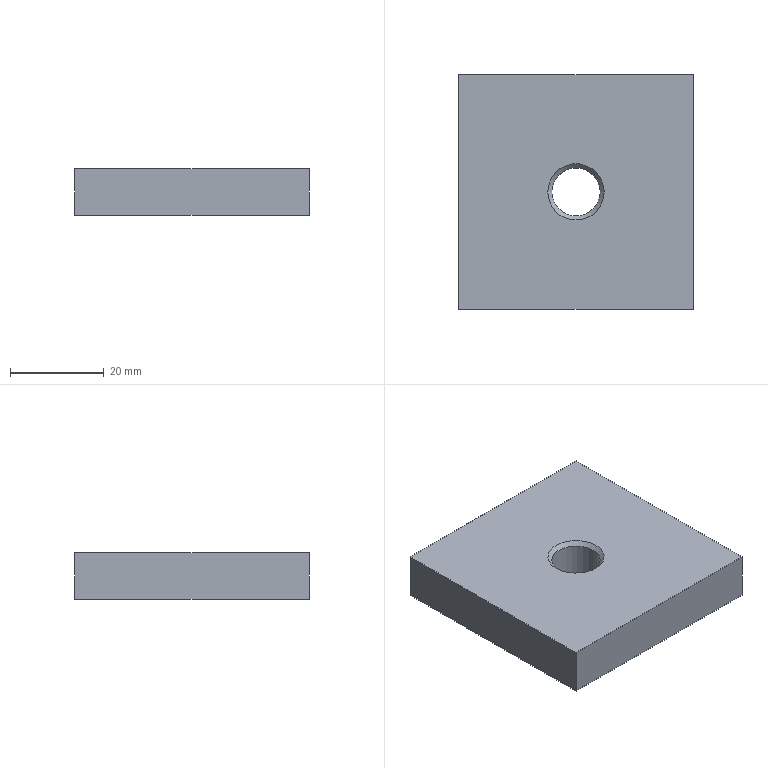Part | STEP file | 冲床-300配套压波_id898_x_t | 1 solid | 9 faces | box 50 x 50 x 10 mm | volume 24142 mm3 | plane 6 | cone 2 | cylinder 1 | commonest cylinder face diameters 10.3 x1
STEP:
#1=CARTESIAN_POINT('',(1160.,230.,-780.));
#2=VERTEX_POINT('',#1);
#3=CARTESIAN_POINT('',(1160.,280.,-780.));
#4=VERTEX_POINT('',#3);
#5=CARTESIAN_POINT('',(1160.,230.,-780.));
#6=DIRECTION('',(0.,1.,0.));
#7=VECTOR('',#6,1.);
#8=LINE('',#5,#7);
#9=EDGE_CURVE('',#2,#4,#8,.T.);
#10=ORIENTED_EDGE('',*,*,#9,.T.);
#11=CARTESIAN_POINT('',(1160.,280.,-790.));
#12=VERTEX_POINT('',#11);
#13=CARTESIAN_POINT('',(1160.,280.,-790.));
#14=DIRECTION('',(0.,0.,1.));
#15=VECTOR('',#14,1.);
#16=LINE('',#13,#15);
#17=EDGE_CURVE('',#12,#4,#16,.T.);
#18=ORIENTED_EDGE('',*,*,#17,.F.);
#19=CARTESIAN_POINT('',(1160.,230.,-790.));
#20=VERTEX_POINT('',#19);
#21=CARTESIAN_POINT('',(1160.,230.,-790.));
#22=DIRECTION('',(0.,1.,0.));
#23=VECTOR('',#22,1.);
#24=LINE('',#21,#23);
#25=EDGE_CURVE('',#20,#12,#24,.T.);
#26=ORIENTED_EDGE('',*,*,#25,.F.);
#27=CARTESIAN_POINT('',(1160.,230.,-790.));
#28=DIRECTION('',(0.,0.,1.));
#29=VECTOR('',#28,1.);
#30=LINE('',#27,#29);
#31=EDGE_CURVE('',#20,#2,#30,.T.);
#32=ORIENTED_EDGE('',*,*,#31,.T.);
#33=EDGE_LOOP('',(#10,#18,#26,#32));
#34=FACE_OUTER_BOUND('',#33,.T.);
#35=CARTESIAN_POINT('',(1160.,230.,-790.));
#36=DIRECTION('',(1.,0.,0.));
#37=DIRECTION('',(0.,0.,1.));
#38=AXIS2_PLACEMENT_3D('',#35,#36,#37);
#39=PLANE('',#38);
#40=ADVANCED_FACE('',(#34),#39,.F.);
#41=CARTESIAN_POINT('',(1210.,280.,-780.));
#42=VERTEX_POINT('',#41);
#43=CARTESIAN_POINT('',(1160.,280.,-780.));
#44=DIRECTION('',(1.,0.,0.));
#45=VECTOR('',#44,1.);
#46=LINE('',#43,#45);
#47=EDGE_CURVE('',#4,#42,#46,.T.);
#48=ORIENTED_EDGE('',*,*,#47,.T.);
#49=CARTESIAN_POINT('',(1210.,280.,-790.));
#50=VERTEX_POINT('',#49);
#51=CARTESIAN_POINT('',(1210.,280.,-790.));
#52=DIRECTION('',(0.,0.,1.));
#53=VECTOR('',#52,1.);
#54=LINE('',#51,#53);
#55=EDGE_CURVE('',#50,#42,#54,.T.);
#56=ORIENTED_EDGE('',*,*,#55,.F.);
#57=CARTESIAN_POINT('',(1160.,280.,-790.));
#58=DIRECTION('',(1.,0.,0.));
#59=VECTOR('',#58,1.);
#60=LINE('',#57,#59);
#61=EDGE_CURVE('',#12,#50,#60,.T.);
#62=ORIENTED_EDGE('',*,*,#61,.F.);
#63=ORIENTED_EDGE('',*,*,#17,.T.);
#64=EDGE_LOOP('',(#48,#56,#62,#63));
#65=FACE_OUTER_BOUND('',#64,.T.);
#66=CARTESIAN_POINT('',(1160.,280.,-790.));
#67=DIRECTION('',(0.,-1.,0.));
#68=DIRECTION('',(0.,0.,-1.));
#69=AXIS2_PLACEMENT_3D('',#66,#67,#68);
#70=PLANE('',#69);
#71=ADVANCED_FACE('',(#65),#70,.F.);
#72=CARTESIAN_POINT('',(1210.,230.,-780.));
#73=VERTEX_POINT('',#72);
#74=CARTESIAN_POINT('',(1210.,280.,-780.));
#75=DIRECTION('',(0.,-1.,0.));
#76=VECTOR('',#75,1.);
#77=LINE('',#74,#76);
#78=EDGE_CURVE('',#42,#73,#77,.T.);
#79=ORIENTED_EDGE('',*,*,#78,.T.);
#80=CARTESIAN_POINT('',(1210.,230.,-790.));
#81=VERTEX_POINT('',#80);
#82=CARTESIAN_POINT('',(1210.,230.,-790.));
#83=DIRECTION('',(0.,0.,1.));
#84=VECTOR('',#83,1.);
#85=LINE('',#82,#84);
#86=EDGE_CURVE('',#81,#73,#85,.T.);
#87=ORIENTED_EDGE('',*,*,#86,.F.);
#88=CARTESIAN_POINT('',(1210.,280.,-790.));
#89=DIRECTION('',(0.,-1.,0.));
#90=VECTOR('',#89,1.);
#91=LINE('',#88,#90);
#92=EDGE_CURVE('',#50,#81,#91,.T.);
#93=ORIENTED_EDGE('',*,*,#92,.F.);
#94=ORIENTED_EDGE('',*,*,#55,.T.);
#95=EDGE_LOOP('',(#79,#87,#93,#94));
#96=FACE_OUTER_BOUND('',#95,.T.);
#97=CARTESIAN_POINT('',(1210.,280.,-790.));
#98=DIRECTION('',(-1.,0.,0.));
#99=DIRECTION('',(0.,0.,-1.));
#100=AXIS2_PLACEMENT_3D('',#97,#98,#99);
#101=PLANE('',#100);
#102=ADVANCED_FACE('',(#96),#101,.F.);
#103=CARTESIAN_POINT('',(1210.,230.,-780.));
#104=DIRECTION('',(-1.,0.,0.));
#105=VECTOR('',#104,1.);
#106=LINE('',#103,#105);
#107=EDGE_CURVE('',#73,#2,#106,.T.);
#108=ORIENTED_EDGE('',*,*,#107,.T.);
#109=ORIENTED_EDGE('',*,*,#31,.F.);
#110=CARTESIAN_POINT('',(1210.,230.,-790.));
#111=DIRECTION('',(-1.,0.,0.));
#112=VECTOR('',#111,1.);
#113=LINE('',#110,#112);
#114=EDGE_CURVE('',#81,#20,#113,.T.);
#115=ORIENTED_EDGE('',*,*,#114,.F.);
#116=ORIENTED_EDGE('',*,*,#86,.T.);
#117=EDGE_LOOP('',(#108,#109,#115,#116));
#118=FACE_OUTER_BOUND('',#117,.T.);
#119=CARTESIAN_POINT('',(1210.,230.,-790.));
#120=DIRECTION('',(0.,1.,0.));
#121=DIRECTION('',(1.,0.,0.));
#122=AXIS2_PLACEMENT_3D('',#119,#120,#121);
#123=PLANE('',#122);
#124=ADVANCED_FACE('',(#118),#123,.F.);
#125=CARTESIAN_POINT('',(1179.,255.,-790.));
#126=VERTEX_POINT('',#125);
#127=CARTESIAN_POINT('',(1185.,255.,-790.));
#128=DIRECTION('',(0.,0.,1.));
#129=DIRECTION('',(-1.,0.,0.));
#130=AXIS2_PLACEMENT_3D('',#127,#128,#129);
#131=CIRCLE('',#130,6.);
#132=EDGE_CURVE('',#126,#126,#131,.T.);
#133=ORIENTED_EDGE('',*,*,#132,.T.);
#134=EDGE_LOOP('',(#133));
#135=FACE_BOUND('',#134,.T.);
#136=ORIENTED_EDGE('',*,*,#25,.T.);
#137=ORIENTED_EDGE('',*,*,#61,.T.);
#138=ORIENTED_EDGE('',*,*,#92,.T.);
#139=ORIENTED_EDGE('',*,*,#114,.T.);
#140=EDGE_LOOP('',(#136,#137,#138,#139));
#141=FACE_BOUND('',#140,.T.);
#142=CARTESIAN_POINT('',(10.,480.,-790.));
#143=DIRECTION('',(0.,0.,-1.));
#144=DIRECTION('',(1.,0.,0.));
#145=AXIS2_PLACEMENT_3D('',#142,#143,#144);
#146=PLANE('',#145);
#147=ADVANCED_FACE('',(#135,#141),#146,.T.);
#148=CARTESIAN_POINT('',(1179.,255.,-780.));
#149=VERTEX_POINT('',#148);
#150=CARTESIAN_POINT('',(1185.,255.,-780.));
#151=DIRECTION('',(0.,0.,-1.));
#152=DIRECTION('',(-1.,0.,0.));
#153=AXIS2_PLACEMENT_3D('',#150,#151,#152);
#154=CIRCLE('',#153,6.);
#155=EDGE_CURVE('',#149,#149,#154,.T.);
#156=ORIENTED_EDGE('',*,*,#155,.T.);
#157=EDGE_LOOP('',(#156));
#158=FACE_BOUND('',#157,.T.);
#159=ORIENTED_EDGE('',*,*,#9,.F.);
#160=ORIENTED_EDGE('',*,*,#107,.F.);
#161=ORIENTED_EDGE('',*,*,#78,.F.);
#162=ORIENTED_EDGE('',*,*,#47,.F.);
#163=EDGE_LOOP('',(#159,#160,#161,#162));
#164=FACE_BOUND('',#163,.T.);
#165=CARTESIAN_POINT('',(10.,480.,-780.));
#166=DIRECTION('',(0.,0.,-1.));
#167=DIRECTION('',(1.,0.,0.));
#168=AXIS2_PLACEMENT_3D('',#165,#166,#167);
#169=PLANE('',#168);
#170=ADVANCED_FACE('',(#158,#164),#169,.F.);
#171=CARTESIAN_POINT('',(1179.85,255.,-780.85));
#172=VERTEX_POINT('',#171);
#173=CARTESIAN_POINT('',(1185.,255.,-780.85));
#174=DIRECTION('',(0.,0.,1.));
#175=DIRECTION('',(-1.,0.,0.));
#176=AXIS2_PLACEMENT_3D('',#173,#174,#175);
#177=CIRCLE('',#176,5.15);
#178=EDGE_CURVE('',#172,#172,#177,.T.);
#179=ORIENTED_EDGE('',*,*,#178,.T.);
#180=EDGE_LOOP('',(#179));
#181=FACE_BOUND('',#180,.T.);
#182=CARTESIAN_POINT('',(1179.85,255.,-789.15));
#183=VERTEX_POINT('',#182);
#184=CARTESIAN_POINT('',(1185.,255.,-789.15));
#185=DIRECTION('',(0.,0.,-1.));
#186=DIRECTION('',(-1.,0.,0.));
#187=AXIS2_PLACEMENT_3D('',#184,#185,#186);
#188=CIRCLE('',#187,5.15);
#189=EDGE_CURVE('',#183,#183,#188,.T.);
#190=ORIENTED_EDGE('',*,*,#189,.T.);
#191=EDGE_LOOP('',(#190));
#192=FACE_BOUND('',#191,.T.);
#193=CARTESIAN_POINT('',(1185.,255.,-790.));
#194=DIRECTION('',(0.,0.,1.));
#195=DIRECTION('',(1.,0.,0.));
#196=AXIS2_PLACEMENT_3D('',#193,#194,#195);
#197=CYLINDRICAL_SURFACE('',#196,5.15);
#198=ADVANCED_FACE('',(#181,#192),#197,.F.);
#199=ORIENTED_EDGE('',*,*,#189,.F.);
#200=EDGE_LOOP('',(#199));
#201=FACE_BOUND('',#200,.T.);
#202=ORIENTED_EDGE('',*,*,#132,.F.);
#203=EDGE_LOOP('',(#202));
#204=FACE_BOUND('',#203,.T.);
#205=CARTESIAN_POINT('',(1185.,255.,-790.));
#206=DIRECTION('',(0.,0.,-1.));
#207=DIRECTION('',(-1.,0.,0.));
#208=AXIS2_PLACEMENT_3D('',#205,#206,#207);
#209=CONICAL_SURFACE('',#208,6.,45.);
#210=ADVANCED_FACE('',(#201,#204),#209,.F.);
#211=ORIENTED_EDGE('',*,*,#178,.F.);
#212=EDGE_LOOP('',(#211));
#213=FACE_BOUND('',#212,.T.);
#214=ORIENTED_EDGE('',*,*,#155,.F.);
#215=EDGE_LOOP('',(#214));
#216=FACE_BOUND('',#215,.T.);
#217=CARTESIAN_POINT('',(1185.,255.,-780.));
#218=DIRECTION('',(0.,0.,1.));
#219=DIRECTION('',(1.,0.,0.));
#220=AXIS2_PLACEMENT_3D('',#217,#218,#219);
#221=CONICAL_SURFACE('',#220,6.,45.);
#222=ADVANCED_FACE('',(#213,#216),#221,.F.);
#223=CLOSED_SHELL('',(#40,#71,#102,#124,#147,#170,#198,#210,#222));
#224=MANIFOLD_SOLID_BREP('',#223);
#225=(LENGTH_UNIT()NAMED_UNIT(*)SI_UNIT(.MILLI.,.METRE.));
#226=UNCERTAINTY_MEASURE_WITH_UNIT(LENGTH_MEASURE(0.00002),#225,'','');
#227=(NAMED_UNIT(*)PLANE_ANGLE_UNIT()SI_UNIT($,.RADIAN.));
#228=PLANE_ANGLE_MEASURE_WITH_UNIT(PLANE_ANGLE_MEASURE(0.01745),#227);
#229=DIMENSIONAL_EXPONENTS(0.,0.,0.,0.,0.,0.,0.);
#230=(CONVERSION_BASED_UNIT('DEGREE',#228)NAMED_UNIT(#229)PLANE_ANGLE_UNIT());
#231=(NAMED_UNIT(*)SI_UNIT($,.STERADIAN.)SOLID_ANGLE_UNIT());
#232=(GEOMETRIC_REPRESENTATION_CONTEXT(3)GLOBAL_UNCERTAINTY_ASSIGNED_CONTEXT((#226))GLOBAL_UNIT_ASSIGNED_CONTEXT((#225,#230,#231))REPRESENTATION_CONTEXT('',''));
#233=ADVANCED_BREP_SHAPE_REPRESENTATION('',(#224),#232);